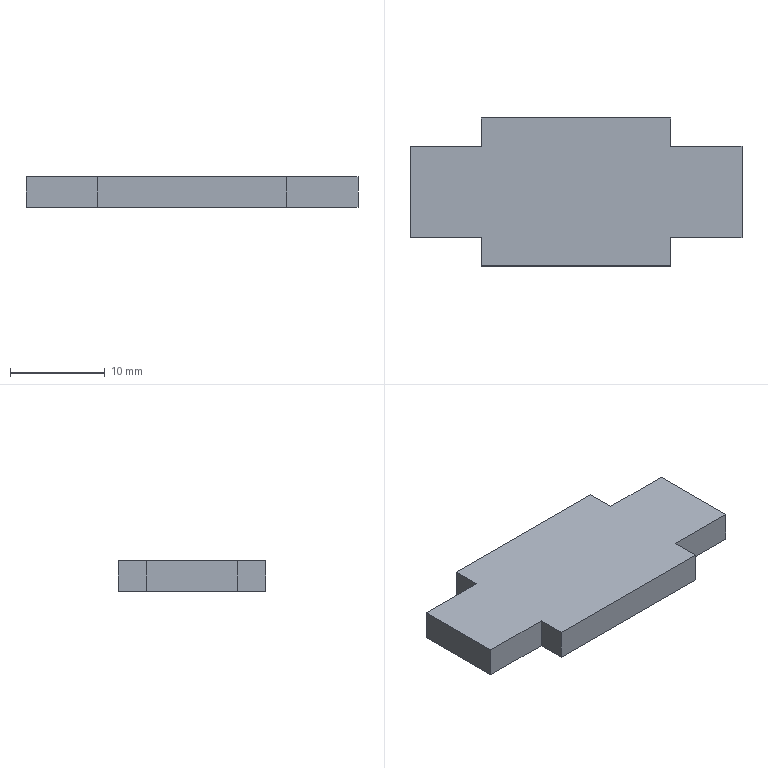Part | SolidWorks | features FlatPattern 1, SMBaseFlange 1, SheetMetal 1 | 1 solid | 14 faces | box 35 x 15.6 x 3.2 mm | volume 1459 mm3 | plane 14
STEP:
#1=CARTESIAN_POINT('',(9.442,-133.501,0.));
#2=VERTEX_POINT('',#1);
#3=CARTESIAN_POINT('',(9.442,-123.901,0.));
#4=VERTEX_POINT('',#3);
#5=CARTESIAN_POINT('',(9.442,-123.901,0.));
#6=DIRECTION('',(0.,1.,0.));
#7=VECTOR('',#6,1000.);
#8=LINE('',#5,#7);
#9=EDGE_CURVE('',#2,#4,#8,.T.);
#10=ORIENTED_EDGE('',*,*,#9,.F.);
#11=CARTESIAN_POINT('',(9.442,-133.501,-3.2));
#12=VERTEX_POINT('',#11);
#13=CARTESIAN_POINT('',(9.442,-133.501,-3.2));
#14=DIRECTION('',(0.,0.,1.));
#15=VECTOR('',#14,1000.);
#16=LINE('',#13,#15);
#17=EDGE_CURVE('',#12,#2,#16,.T.);
#18=ORIENTED_EDGE('',*,*,#17,.F.);
#19=CARTESIAN_POINT('',(9.442,-123.901,-3.2));
#20=VERTEX_POINT('',#19);
#21=CARTESIAN_POINT('',(9.442,-123.901,-3.2));
#22=DIRECTION('',(0.,1.,0.));
#23=VECTOR('',#22,1000.);
#24=LINE('',#21,#23);
#25=EDGE_CURVE('',#12,#20,#24,.T.);
#26=ORIENTED_EDGE('',*,*,#25,.T.);
#27=CARTESIAN_POINT('',(9.442,-123.901,-3.2));
#28=DIRECTION('',(0.,0.,1.));
#29=VECTOR('',#28,1000.);
#30=LINE('',#27,#29);
#31=EDGE_CURVE('',#20,#4,#30,.T.);
#32=ORIENTED_EDGE('',*,*,#31,.T.);
#33=EDGE_LOOP('',(#10,#18,#26,#32));
#34=FACE_OUTER_BOUND('',#33,.T.);
#35=CARTESIAN_POINT('',(9.442,-123.901,-3.2));
#36=DIRECTION('',(1.,0.,0.));
#37=DIRECTION('',(0.,1.,0.));
#38=AXIS2_PLACEMENT_3D('',#35,#36,#37);
#39=PLANE('',#38);
#40=ADVANCED_FACE('',(#34),#39,.T.);
#41=CARTESIAN_POINT('',(1.942,-133.501,0.));
#42=VERTEX_POINT('',#41);
#43=CARTESIAN_POINT('',(9.442,-133.501,0.));
#44=DIRECTION('',(1.,0.,0.));
#45=VECTOR('',#44,1000.);
#46=LINE('',#43,#45);
#47=EDGE_CURVE('',#42,#2,#46,.T.);
#48=ORIENTED_EDGE('',*,*,#47,.F.);
#49=CARTESIAN_POINT('',(1.942,-133.501,-3.2));
#50=VERTEX_POINT('',#49);
#51=CARTESIAN_POINT('',(1.942,-133.501,-3.2));
#52=DIRECTION('',(0.,0.,1.));
#53=VECTOR('',#52,1000.);
#54=LINE('',#51,#53);
#55=EDGE_CURVE('',#50,#42,#54,.T.);
#56=ORIENTED_EDGE('',*,*,#55,.F.);
#57=CARTESIAN_POINT('',(9.442,-133.501,-3.2));
#58=DIRECTION('',(1.,0.,0.));
#59=VECTOR('',#58,1000.);
#60=LINE('',#57,#59);
#61=EDGE_CURVE('',#50,#12,#60,.T.);
#62=ORIENTED_EDGE('',*,*,#61,.T.);
#63=ORIENTED_EDGE('',*,*,#17,.T.);
#64=EDGE_LOOP('',(#48,#56,#62,#63));
#65=FACE_OUTER_BOUND('',#64,.T.);
#66=CARTESIAN_POINT('',(9.442,-133.501,-3.2));
#67=DIRECTION('',(0.,-1.,0.));
#68=DIRECTION('',(0.,0.,-1.));
#69=AXIS2_PLACEMENT_3D('',#66,#67,#68);
#70=PLANE('',#69);
#71=ADVANCED_FACE('',(#65),#70,.T.);
#72=CARTESIAN_POINT('',(1.942,-136.501,0.));
#73=VERTEX_POINT('',#72);
#74=CARTESIAN_POINT('',(1.942,-133.501,0.));
#75=DIRECTION('',(0.,1.,0.));
#76=VECTOR('',#75,1000.);
#77=LINE('',#74,#76);
#78=EDGE_CURVE('',#73,#42,#77,.T.);
#79=ORIENTED_EDGE('',*,*,#78,.F.);
#80=CARTESIAN_POINT('',(1.942,-136.501,-3.2));
#81=VERTEX_POINT('',#80);
#82=CARTESIAN_POINT('',(1.942,-136.501,-3.2));
#83=DIRECTION('',(0.,0.,1.));
#84=VECTOR('',#83,1000.);
#85=LINE('',#82,#84);
#86=EDGE_CURVE('',#81,#73,#85,.T.);
#87=ORIENTED_EDGE('',*,*,#86,.F.);
#88=CARTESIAN_POINT('',(1.942,-133.501,-3.2));
#89=DIRECTION('',(0.,1.,0.));
#90=VECTOR('',#89,1000.);
#91=LINE('',#88,#90);
#92=EDGE_CURVE('',#81,#50,#91,.T.);
#93=ORIENTED_EDGE('',*,*,#92,.T.);
#94=ORIENTED_EDGE('',*,*,#55,.T.);
#95=EDGE_LOOP('',(#79,#87,#93,#94));
#96=FACE_OUTER_BOUND('',#95,.T.);
#97=CARTESIAN_POINT('',(1.942,-133.501,-3.2));
#98=DIRECTION('',(1.,0.,0.));
#99=DIRECTION('',(0.,1.,0.));
#100=AXIS2_PLACEMENT_3D('',#97,#98,#99);
#101=PLANE('',#100);
#102=ADVANCED_FACE('',(#96),#101,.T.);
#103=CARTESIAN_POINT('',(-18.058,-136.501,0.));
#104=VERTEX_POINT('',#103);
#105=CARTESIAN_POINT('',(1.942,-136.501,0.));
#106=DIRECTION('',(1.,0.,0.));
#107=VECTOR('',#106,1000.);
#108=LINE('',#105,#107);
#109=EDGE_CURVE('',#104,#73,#108,.T.);
#110=ORIENTED_EDGE('',*,*,#109,.F.);
#111=CARTESIAN_POINT('',(-18.058,-136.501,-3.2));
#112=VERTEX_POINT('',#111);
#113=CARTESIAN_POINT('',(-18.058,-136.501,-3.2));
#114=DIRECTION('',(0.,0.,1.));
#115=VECTOR('',#114,1000.);
#116=LINE('',#113,#115);
#117=EDGE_CURVE('',#112,#104,#116,.T.);
#118=ORIENTED_EDGE('',*,*,#117,.F.);
#119=CARTESIAN_POINT('',(1.942,-136.501,-3.2));
#120=DIRECTION('',(1.,0.,0.));
#121=VECTOR('',#120,1000.);
#122=LINE('',#119,#121);
#123=EDGE_CURVE('',#112,#81,#122,.T.);
#124=ORIENTED_EDGE('',*,*,#123,.T.);
#125=ORIENTED_EDGE('',*,*,#86,.T.);
#126=EDGE_LOOP('',(#110,#118,#124,#125));
#127=FACE_OUTER_BOUND('',#126,.T.);
#128=CARTESIAN_POINT('',(1.942,-136.501,-3.2));
#129=DIRECTION('',(0.,-1.,0.));
#130=DIRECTION('',(0.,0.,-1.));
#131=AXIS2_PLACEMENT_3D('',#128,#129,#130);
#132=PLANE('',#131);
#133=ADVANCED_FACE('',(#127),#132,.T.);
#134=CARTESIAN_POINT('',(-18.058,-133.501,0.));
#135=VERTEX_POINT('',#134);
#136=CARTESIAN_POINT('',(-18.058,-136.501,0.));
#137=DIRECTION('',(0.,-1.,0.));
#138=VECTOR('',#137,1000.);
#139=LINE('',#136,#138);
#140=EDGE_CURVE('',#135,#104,#139,.T.);
#141=ORIENTED_EDGE('',*,*,#140,.F.);
#142=CARTESIAN_POINT('',(-18.058,-133.501,-3.2));
#143=VERTEX_POINT('',#142);
#144=CARTESIAN_POINT('',(-18.058,-133.501,-3.2));
#145=DIRECTION('',(0.,0.,1.));
#146=VECTOR('',#145,1000.);
#147=LINE('',#144,#146);
#148=EDGE_CURVE('',#143,#135,#147,.T.);
#149=ORIENTED_EDGE('',*,*,#148,.F.);
#150=CARTESIAN_POINT('',(-18.058,-136.501,-3.2));
#151=DIRECTION('',(0.,-1.,0.));
#152=VECTOR('',#151,1000.);
#153=LINE('',#150,#152);
#154=EDGE_CURVE('',#143,#112,#153,.T.);
#155=ORIENTED_EDGE('',*,*,#154,.T.);
#156=ORIENTED_EDGE('',*,*,#117,.T.);
#157=EDGE_LOOP('',(#141,#149,#155,#156));
#158=FACE_OUTER_BOUND('',#157,.T.);
#159=CARTESIAN_POINT('',(-18.058,-136.501,-3.2));
#160=DIRECTION('',(-1.,0.,0.));
#161=DIRECTION('',(0.,-1.,0.));
#162=AXIS2_PLACEMENT_3D('',#159,#160,#161);
#163=PLANE('',#162);
#164=ADVANCED_FACE('',(#158),#163,.T.);
#165=CARTESIAN_POINT('',(-25.558,-133.501,0.));
#166=VERTEX_POINT('',#165);
#167=CARTESIAN_POINT('',(-18.058,-133.501,0.));
#168=DIRECTION('',(1.,0.,0.));
#169=VECTOR('',#168,1000.);
#170=LINE('',#167,#169);
#171=EDGE_CURVE('',#166,#135,#170,.T.);
#172=ORIENTED_EDGE('',*,*,#171,.F.);
#173=CARTESIAN_POINT('',(-25.558,-133.501,-3.2));
#174=VERTEX_POINT('',#173);
#175=CARTESIAN_POINT('',(-25.558,-133.501,-3.2));
#176=DIRECTION('',(0.,0.,1.));
#177=VECTOR('',#176,1000.);
#178=LINE('',#175,#177);
#179=EDGE_CURVE('',#174,#166,#178,.T.);
#180=ORIENTED_EDGE('',*,*,#179,.F.);
#181=CARTESIAN_POINT('',(-18.058,-133.501,-3.2));
#182=DIRECTION('',(1.,0.,0.));
#183=VECTOR('',#182,1000.);
#184=LINE('',#181,#183);
#185=EDGE_CURVE('',#174,#143,#184,.T.);
#186=ORIENTED_EDGE('',*,*,#185,.T.);
#187=ORIENTED_EDGE('',*,*,#148,.T.);
#188=EDGE_LOOP('',(#172,#180,#186,#187));
#189=FACE_OUTER_BOUND('',#188,.T.);
#190=CARTESIAN_POINT('',(-18.058,-133.501,-3.2));
#191=DIRECTION('',(0.,-1.,0.));
#192=DIRECTION('',(0.,0.,-1.));
#193=AXIS2_PLACEMENT_3D('',#190,#191,#192);
#194=PLANE('',#193);
#195=ADVANCED_FACE('',(#189),#194,.T.);
#196=CARTESIAN_POINT('',(-25.558,-123.901,0.));
#197=VERTEX_POINT('',#196);
#198=CARTESIAN_POINT('',(-25.558,-123.901,0.));
#199=DIRECTION('',(0.,-1.,0.));
#200=VECTOR('',#199,1000.);
#201=LINE('',#198,#200);
#202=EDGE_CURVE('',#197,#166,#201,.T.);
#203=ORIENTED_EDGE('',*,*,#202,.F.);
#204=CARTESIAN_POINT('',(-25.558,-123.901,-3.2));
#205=VERTEX_POINT('',#204);
#206=CARTESIAN_POINT('',(-25.558,-123.901,-3.2));
#207=DIRECTION('',(0.,0.,1.));
#208=VECTOR('',#207,1000.);
#209=LINE('',#206,#208);
#210=EDGE_CURVE('',#205,#197,#209,.T.);
#211=ORIENTED_EDGE('',*,*,#210,.F.);
#212=CARTESIAN_POINT('',(-25.558,-123.901,-3.2));
#213=DIRECTION('',(0.,-1.,0.));
#214=VECTOR('',#213,1000.);
#215=LINE('',#212,#214);
#216=EDGE_CURVE('',#205,#174,#215,.T.);
#217=ORIENTED_EDGE('',*,*,#216,.T.);
#218=ORIENTED_EDGE('',*,*,#179,.T.);
#219=EDGE_LOOP('',(#203,#211,#217,#218));
#220=FACE_OUTER_BOUND('',#219,.T.);
#221=CARTESIAN_POINT('',(-25.558,-123.901,-3.2));
#222=DIRECTION('',(-1.,0.,0.));
#223=DIRECTION('',(0.,0.,1.));
#224=AXIS2_PLACEMENT_3D('',#221,#222,#223);
#225=PLANE('',#224);
#226=ADVANCED_FACE('',(#220),#225,.T.);
#227=CARTESIAN_POINT('',(-18.058,-123.901,0.));
#228=VERTEX_POINT('',#227);
#229=CARTESIAN_POINT('',(-18.058,-123.901,0.));
#230=DIRECTION('',(-1.,0.,0.));
#231=VECTOR('',#230,1000.);
#232=LINE('',#229,#231);
#233=EDGE_CURVE('',#228,#197,#232,.T.);
#234=ORIENTED_EDGE('',*,*,#233,.F.);
#235=CARTESIAN_POINT('',(-18.058,-123.901,-3.2));
#236=VERTEX_POINT('',#235);
#237=CARTESIAN_POINT('',(-18.058,-123.901,-3.2));
#238=DIRECTION('',(0.,0.,1.));
#239=VECTOR('',#238,1000.);
#240=LINE('',#237,#239);
#241=EDGE_CURVE('',#236,#228,#240,.T.);
#242=ORIENTED_EDGE('',*,*,#241,.F.);
#243=CARTESIAN_POINT('',(-18.058,-123.901,-3.2));
#244=DIRECTION('',(-1.,0.,0.));
#245=VECTOR('',#244,1000.);
#246=LINE('',#243,#245);
#247=EDGE_CURVE('',#236,#205,#246,.T.);
#248=ORIENTED_EDGE('',*,*,#247,.T.);
#249=ORIENTED_EDGE('',*,*,#210,.T.);
#250=EDGE_LOOP('',(#234,#242,#248,#249));
#251=FACE_OUTER_BOUND('',#250,.T.);
#252=CARTESIAN_POINT('',(-18.058,-123.901,-3.2));
#253=DIRECTION('',(0.,1.,0.));
#254=DIRECTION('',(0.,0.,1.));
#255=AXIS2_PLACEMENT_3D('',#252,#253,#254);
#256=PLANE('',#255);
#257=ADVANCED_FACE('',(#251),#256,.T.);
#258=CARTESIAN_POINT('',(-18.058,-120.901,0.));
#259=VERTEX_POINT('',#258);
#260=CARTESIAN_POINT('',(-18.058,-120.901,0.));
#261=DIRECTION('',(0.,-1.,0.));
#262=VECTOR('',#261,1000.);
#263=LINE('',#260,#262);
#264=EDGE_CURVE('',#259,#228,#263,.T.);
#265=ORIENTED_EDGE('',*,*,#264,.F.);
#266=CARTESIAN_POINT('',(-18.058,-120.901,-3.2));
#267=VERTEX_POINT('',#266);
#268=CARTESIAN_POINT('',(-18.058,-120.901,-3.2));
#269=DIRECTION('',(0.,0.,1.));
#270=VECTOR('',#269,1000.);
#271=LINE('',#268,#270);
#272=EDGE_CURVE('',#267,#259,#271,.T.);
#273=ORIENTED_EDGE('',*,*,#272,.F.);
#274=CARTESIAN_POINT('',(-18.058,-120.901,-3.2));
#275=DIRECTION('',(0.,-1.,0.));
#276=VECTOR('',#275,1000.);
#277=LINE('',#274,#276);
#278=EDGE_CURVE('',#267,#236,#277,.T.);
#279=ORIENTED_EDGE('',*,*,#278,.T.);
#280=ORIENTED_EDGE('',*,*,#241,.T.);
#281=EDGE_LOOP('',(#265,#273,#279,#280));
#282=FACE_OUTER_BOUND('',#281,.T.);
#283=CARTESIAN_POINT('',(-18.058,-120.901,-3.2));
#284=DIRECTION('',(-1.,0.,0.));
#285=DIRECTION('',(0.,0.,1.));
#286=AXIS2_PLACEMENT_3D('',#283,#284,#285);
#287=PLANE('',#286);
#288=ADVANCED_FACE('',(#282),#287,.T.);
#289=CARTESIAN_POINT('',(1.942,-120.901,0.));
#290=VERTEX_POINT('',#289);
#291=CARTESIAN_POINT('',(1.942,-120.901,0.));
#292=DIRECTION('',(-1.,0.,0.));
#293=VECTOR('',#292,1000.);
#294=LINE('',#291,#293);
#295=EDGE_CURVE('',#290,#259,#294,.T.);
#296=ORIENTED_EDGE('',*,*,#295,.F.);
#297=CARTESIAN_POINT('',(1.942,-120.901,-3.2));
#298=VERTEX_POINT('',#297);
#299=CARTESIAN_POINT('',(1.942,-120.901,-3.2));
#300=DIRECTION('',(0.,0.,1.));
#301=VECTOR('',#300,1000.);
#302=LINE('',#299,#301);
#303=EDGE_CURVE('',#298,#290,#302,.T.);
#304=ORIENTED_EDGE('',*,*,#303,.F.);
#305=CARTESIAN_POINT('',(1.942,-120.901,-3.2));
#306=DIRECTION('',(-1.,0.,0.));
#307=VECTOR('',#306,1000.);
#308=LINE('',#305,#307);
#309=EDGE_CURVE('',#298,#267,#308,.T.);
#310=ORIENTED_EDGE('',*,*,#309,.T.);
#311=ORIENTED_EDGE('',*,*,#272,.T.);
#312=EDGE_LOOP('',(#296,#304,#310,#311));
#313=FACE_OUTER_BOUND('',#312,.T.);
#314=CARTESIAN_POINT('',(1.942,-120.901,-3.2));
#315=DIRECTION('',(0.,1.,0.));
#316=DIRECTION('',(0.,0.,1.));
#317=AXIS2_PLACEMENT_3D('',#314,#315,#316);
#318=PLANE('',#317);
#319=ADVANCED_FACE('',(#313),#318,.T.);
#320=CARTESIAN_POINT('',(1.942,-123.901,0.));
#321=VERTEX_POINT('',#320);
#322=CARTESIAN_POINT('',(1.942,-123.901,0.));
#323=DIRECTION('',(0.,1.,0.));
#324=VECTOR('',#323,1000.);
#325=LINE('',#322,#324);
#326=EDGE_CURVE('',#321,#290,#325,.T.);
#327=ORIENTED_EDGE('',*,*,#326,.F.);
#328=CARTESIAN_POINT('',(1.942,-123.901,-3.2));
#329=VERTEX_POINT('',#328);
#330=CARTESIAN_POINT('',(1.942,-123.901,-3.2));
#331=DIRECTION('',(0.,0.,1.));
#332=VECTOR('',#331,1000.);
#333=LINE('',#330,#332);
#334=EDGE_CURVE('',#329,#321,#333,.T.);
#335=ORIENTED_EDGE('',*,*,#334,.F.);
#336=CARTESIAN_POINT('',(1.942,-123.901,-3.2));
#337=DIRECTION('',(0.,1.,0.));
#338=VECTOR('',#337,1000.);
#339=LINE('',#336,#338);
#340=EDGE_CURVE('',#329,#298,#339,.T.);
#341=ORIENTED_EDGE('',*,*,#340,.T.);
#342=ORIENTED_EDGE('',*,*,#303,.T.);
#343=EDGE_LOOP('',(#327,#335,#341,#342));
#344=FACE_OUTER_BOUND('',#343,.T.);
#345=CARTESIAN_POINT('',(1.942,-123.901,-3.2));
#346=DIRECTION('',(1.,0.,0.));
#347=DIRECTION('',(0.,0.,-1.));
#348=AXIS2_PLACEMENT_3D('',#345,#346,#347);
#349=PLANE('',#348);
#350=ADVANCED_FACE('',(#344),#349,.T.);
#351=CARTESIAN_POINT('',(9.442,-123.901,0.));
#352=DIRECTION('',(-1.,0.,0.));
#353=VECTOR('',#352,1000.);
#354=LINE('',#351,#353);
#355=EDGE_CURVE('',#4,#321,#354,.T.);
#356=ORIENTED_EDGE('',*,*,#355,.F.);
#357=ORIENTED_EDGE('',*,*,#31,.F.);
#358=CARTESIAN_POINT('',(9.442,-123.901,-3.2));
#359=DIRECTION('',(-1.,0.,0.));
#360=VECTOR('',#359,1000.);
#361=LINE('',#358,#360);
#362=EDGE_CURVE('',#20,#329,#361,.T.);
#363=ORIENTED_EDGE('',*,*,#362,.T.);
#364=ORIENTED_EDGE('',*,*,#334,.T.);
#365=EDGE_LOOP('',(#356,#357,#363,#364));
#366=FACE_OUTER_BOUND('',#365,.T.);
#367=CARTESIAN_POINT('',(9.442,-123.901,-3.2));
#368=DIRECTION('',(0.,1.,0.));
#369=DIRECTION('',(0.,0.,1.));
#370=AXIS2_PLACEMENT_3D('',#367,#368,#369);
#371=PLANE('',#370);
#372=ADVANCED_FACE('',(#366),#371,.T.);
#373=ORIENTED_EDGE('',*,*,#25,.F.);
#374=ORIENTED_EDGE('',*,*,#61,.F.);
#375=ORIENTED_EDGE('',*,*,#92,.F.);
#376=ORIENTED_EDGE('',*,*,#123,.F.);
#377=ORIENTED_EDGE('',*,*,#154,.F.);
#378=ORIENTED_EDGE('',*,*,#185,.F.);
#379=ORIENTED_EDGE('',*,*,#216,.F.);
#380=ORIENTED_EDGE('',*,*,#247,.F.);
#381=ORIENTED_EDGE('',*,*,#278,.F.);
#382=ORIENTED_EDGE('',*,*,#309,.F.);
#383=ORIENTED_EDGE('',*,*,#340,.F.);
#384=ORIENTED_EDGE('',*,*,#362,.F.);
#385=EDGE_LOOP('',(#373,#374,#375,#376,#377,#378,#379,#380,#381,#382,#383,#384));
#386=FACE_OUTER_BOUND('',#385,.T.);
#387=CARTESIAN_POINT('',(0.,0.,-3.2));
#388=DIRECTION('',(0.,0.,-1.));
#389=DIRECTION('',(-1.,0.,0.));
#390=AXIS2_PLACEMENT_3D('',#387,#388,#389);
#391=PLANE('',#390);
#392=ADVANCED_FACE('',(#386),#391,.T.);
#393=ORIENTED_EDGE('',*,*,#9,.T.);
#394=ORIENTED_EDGE('',*,*,#355,.T.);
#395=ORIENTED_EDGE('',*,*,#326,.T.);
#396=ORIENTED_EDGE('',*,*,#295,.T.);
#397=ORIENTED_EDGE('',*,*,#264,.T.);
#398=ORIENTED_EDGE('',*,*,#233,.T.);
#399=ORIENTED_EDGE('',*,*,#202,.T.);
#400=ORIENTED_EDGE('',*,*,#171,.T.);
#401=ORIENTED_EDGE('',*,*,#140,.T.);
#402=ORIENTED_EDGE('',*,*,#109,.T.);
#403=ORIENTED_EDGE('',*,*,#78,.T.);
#404=ORIENTED_EDGE('',*,*,#47,.T.);
#405=EDGE_LOOP('',(#393,#394,#395,#396,#397,#398,#399,#400,#401,#402,#403,#404));
#406=FACE_OUTER_BOUND('',#405,.T.);
#407=CARTESIAN_POINT('',(0.,0.,0.));
#408=DIRECTION('',(0.,0.,-1.));
#409=DIRECTION('',(-1.,0.,0.));
#410=AXIS2_PLACEMENT_3D('',#407,#408,#409);
#411=PLANE('',#410);
#412=ADVANCED_FACE('',(#406),#411,.F.);
#413=CLOSED_SHELL('',(#40,#71,#102,#133,#164,#195,#226,#257,#288,#319,#350,#372,#392,#412));
#414=MANIFOLD_SOLID_BREP('',#413);
#415=CARTESIAN_POINT('',(0.,0.,0.));
#416=DIRECTION('',(0.,0.,1.));
#417=DIRECTION('',(1.,0.,0.));
#418=AXIS2_PLACEMENT_3D('',#415,#416,#417);
#419=(LENGTH_UNIT()NAMED_UNIT(*)SI_UNIT(.MILLI.,.METRE.));
#420=UNCERTAINTY_MEASURE_WITH_UNIT(LENGTH_MEASURE(0.00001),#419,'','');
#421=(NAMED_UNIT(*)PLANE_ANGLE_UNIT()SI_UNIT($,.RADIAN.));
#422=(NAMED_UNIT(*)SI_UNIT($,.STERADIAN.)SOLID_ANGLE_UNIT());
#423=(GEOMETRIC_REPRESENTATION_CONTEXT(3)GLOBAL_UNCERTAINTY_ASSIGNED_CONTEXT((#420))GLOBAL_UNIT_ASSIGNED_CONTEXT((#419,#421,#422))REPRESENTATION_CONTEXT('',''));
#424=ADVANCED_BREP_SHAPE_REPRESENTATION('',(#414,#418),#423);